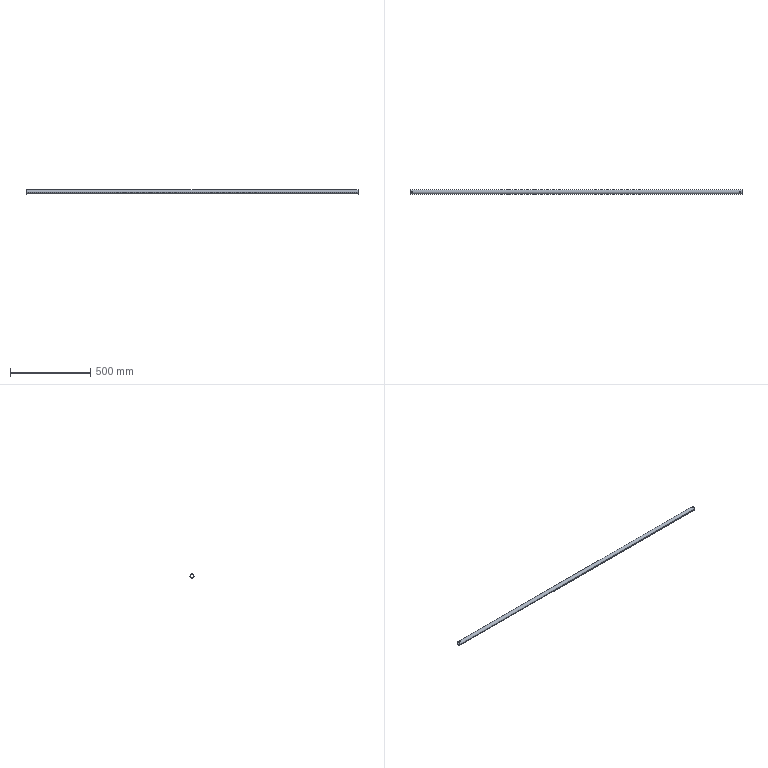Part | NX | features BREP 1 | 1 solid | 10 faces | box 2065 x 25.4 x 25.4 mm | volume 191174 mm3 | cylinder 8 | plane 2 | commonest cylinder face diameters 6.604 x4 22.962 x2 25.4 x2
STEP:
#1=CARTESIAN_POINT('',(-1032.51,12.7,0.));
#2=VERTEX_POINT('',#1);
#3=CARTESIAN_POINT('',(-1032.51,-12.7,0.));
#4=VERTEX_POINT('',#3);
#5=CARTESIAN_POINT('',(-1032.51,0.,0.));
#6=DIRECTION('',(1.,0.,0.));
#7=DIRECTION('',(0.,1.,0.));
#8=AXIS2_PLACEMENT_3D('',#5,#6,#7);
#9=CIRCLE('',#8,12.7);
#10=EDGE_CURVE('',#2,#4,#9,.T.);
#11=ORIENTED_EDGE('',*,*,#10,.F.);
#12=CARTESIAN_POINT('',(-1032.51,0.,0.));
#13=DIRECTION('',(1.,0.,0.));
#14=DIRECTION('',(0.,-1.,0.));
#15=AXIS2_PLACEMENT_3D('',#12,#13,#14);
#16=CIRCLE('',#15,12.7);
#17=EDGE_CURVE('',#4,#2,#16,.T.);
#18=ORIENTED_EDGE('',*,*,#17,.F.);
#19=EDGE_LOOP('',(#11,#18));
#20=FACE_BOUND('',#19,.T.);
#21=CARTESIAN_POINT('',(-1032.51,11.481,0.));
#22=VERTEX_POINT('',#21);
#23=CARTESIAN_POINT('',(-1032.51,-11.481,0.));
#24=VERTEX_POINT('',#23);
#25=CARTESIAN_POINT('',(-1032.51,0.,0.));
#26=DIRECTION('',(-1.,0.,0.));
#27=DIRECTION('',(0.,1.,0.));
#28=AXIS2_PLACEMENT_3D('',#25,#26,#27);
#29=CIRCLE('',#28,11.481);
#30=EDGE_CURVE('',#22,#24,#29,.T.);
#31=ORIENTED_EDGE('',*,*,#30,.F.);
#32=CARTESIAN_POINT('',(-1032.51,0.,0.));
#33=DIRECTION('',(-1.,0.,0.));
#34=DIRECTION('',(0.,-1.,0.));
#35=AXIS2_PLACEMENT_3D('',#32,#33,#34);
#36=CIRCLE('',#35,11.481);
#37=EDGE_CURVE('',#24,#22,#36,.T.);
#38=ORIENTED_EDGE('',*,*,#37,.F.);
#39=EDGE_LOOP('',(#31,#38));
#40=FACE_BOUND('',#39,.T.);
#41=CARTESIAN_POINT('',(-1032.51,0.,0.));
#42=DIRECTION('',(1.,0.,0.));
#43=DIRECTION('',(0.,1.,0.));
#44=AXIS2_PLACEMENT_3D('',#41,#42,#43);
#45=PLANE('',#44);
#46=ADVANCED_FACE('',(#20,#40),#45,.F.);
#47=CARTESIAN_POINT('',(1032.51,12.7,0.));
#48=VERTEX_POINT('',#47);
#49=CARTESIAN_POINT('',(-1032.51,12.7,0.));
#50=DIRECTION('',(1.,0.,0.));
#51=VECTOR('',#50,1000.);
#52=LINE('',#49,#51);
#53=EDGE_CURVE('',#48,#2,#52,.F.);
#54=ORIENTED_EDGE('',*,*,#53,.F.);
#55=CARTESIAN_POINT('',(1032.51,-12.7,0.));
#56=VERTEX_POINT('',#55);
#57=CARTESIAN_POINT('',(1032.51,0.,0.));
#58=DIRECTION('',(1.,0.,0.));
#59=DIRECTION('',(0.,-1.,0.));
#60=AXIS2_PLACEMENT_3D('',#57,#58,#59);
#61=CIRCLE('',#60,12.7);
#62=EDGE_CURVE('',#56,#48,#61,.T.);
#63=ORIENTED_EDGE('',*,*,#62,.F.);
#64=CARTESIAN_POINT('',(-1032.51,-12.7,0.));
#65=DIRECTION('',(1.,0.,0.));
#66=VECTOR('',#65,1000.);
#67=LINE('',#64,#66);
#68=EDGE_CURVE('',#56,#4,#67,.F.);
#69=ORIENTED_EDGE('',*,*,#68,.T.);
#70=ORIENTED_EDGE('',*,*,#17,.T.);
#71=EDGE_LOOP('',(#54,#63,#69,#70));
#72=FACE_BOUND('',#71,.T.);
#73=CARTESIAN_POINT('',(-1032.51,0.,0.));
#74=DIRECTION('',(1.,0.,0.));
#75=DIRECTION('',(0.,-1.,0.));
#76=AXIS2_PLACEMENT_3D('',#73,#74,#75);
#77=CYLINDRICAL_SURFACE('',#76,12.7);
#78=ADVANCED_FACE('',(#72),#77,.T.);
#79=ORIENTED_EDGE('',*,*,#68,.F.);
#80=CARTESIAN_POINT('',(1032.51,0.,0.));
#81=DIRECTION('',(1.,0.,0.));
#82=DIRECTION('',(0.,1.,0.));
#83=AXIS2_PLACEMENT_3D('',#80,#81,#82);
#84=CIRCLE('',#83,12.7);
#85=EDGE_CURVE('',#48,#56,#84,.T.);
#86=ORIENTED_EDGE('',*,*,#85,.F.);
#87=ORIENTED_EDGE('',*,*,#53,.T.);
#88=ORIENTED_EDGE('',*,*,#10,.T.);
#89=EDGE_LOOP('',(#79,#86,#87,#88));
#90=FACE_BOUND('',#89,.T.);
#91=CARTESIAN_POINT('',(1023.112,0.,12.7));
#92=VERTEX_POINT('',#91);
#93=CARTESIAN_POINT('',(1016.508,0.,12.7));
#94=VERTEX_POINT('',#93);
#95=CARTESIAN_POINT('',(1023.112,0.,12.7));
#96=CARTESIAN_POINT('',(1023.112,-0.4503,12.7));
#97=CARTESIAN_POINT('',(1022.958,-1.282,12.655));
#98=CARTESIAN_POINT('',(1021.952,-2.768,12.426));
#99=CARTESIAN_POINT('',(1019.831,-3.655,12.156));
#100=CARTESIAN_POINT('',(1017.67,-2.773,12.425));
#101=CARTESIAN_POINT('',(1016.664,-1.286,12.654));
#102=CARTESIAN_POINT('',(1016.508,-0.4521,12.7));
#103=CARTESIAN_POINT('',(1016.508,0.,12.7));
#104=B_SPLINE_CURVE_WITH_KNOTS('',3,(#95,#96,#97,#98,#99,#100,#101,#102,#103),.UNSPECIFIED.,.F.,.F.,(4,1,1,1,1,1,4),(0.,0.125,0.25,0.5,0.75,0.875,1.),.UNSPECIFIED.);
#105=EDGE_CURVE('',#92,#94,#104,.T.);
#106=ORIENTED_EDGE('',*,*,#105,.T.);
#107=CARTESIAN_POINT('',(1016.508,0.,12.7));
#108=CARTESIAN_POINT('',(1016.508,0.4503,12.7));
#109=CARTESIAN_POINT('',(1016.662,1.282,12.655));
#110=CARTESIAN_POINT('',(1017.668,2.768,12.426));
#111=CARTESIAN_POINT('',(1019.789,3.655,12.156));
#112=CARTESIAN_POINT('',(1021.95,2.773,12.425));
#113=CARTESIAN_POINT('',(1022.956,1.286,12.654));
#114=CARTESIAN_POINT('',(1023.112,0.4521,12.7));
#115=CARTESIAN_POINT('',(1023.112,0.,12.7));
#116=B_SPLINE_CURVE_WITH_KNOTS('',3,(#107,#108,#109,#110,#111,#112,#113,#114,#115),.UNSPECIFIED.,.F.,.F.,(4,1,1,1,1,1,4),(0.,0.125,0.25,0.5,0.75,0.875,1.),.UNSPECIFIED.);
#117=EDGE_CURVE('',#94,#92,#116,.T.);
#118=ORIENTED_EDGE('',*,*,#117,.T.);
#119=EDGE_LOOP('',(#106,#118));
#120=FACE_BOUND('',#119,.T.);
#121=CARTESIAN_POINT('',(-1016.508,0.,12.7));
#122=VERTEX_POINT('',#121);
#123=CARTESIAN_POINT('',(-1023.112,0.,12.7));
#124=VERTEX_POINT('',#123);
#125=CARTESIAN_POINT('',(-1016.508,0.,12.7));
#126=CARTESIAN_POINT('',(-1016.508,-0.4517,12.7));
#127=CARTESIAN_POINT('',(-1016.664,-1.285,12.654));
#128=CARTESIAN_POINT('',(-1017.67,-2.774,12.425));
#129=CARTESIAN_POINT('',(-1019.831,-3.655,12.156));
#130=CARTESIAN_POINT('',(-1021.952,-2.767,12.426));
#131=CARTESIAN_POINT('',(-1022.958,-1.282,12.655));
#132=CARTESIAN_POINT('',(-1023.112,-0.4506,12.7));
#133=CARTESIAN_POINT('',(-1023.112,0.,12.7));
#134=B_SPLINE_CURVE_WITH_KNOTS('',3,(#125,#126,#127,#128,#129,#130,#131,#132,#133),.UNSPECIFIED.,.F.,.F.,(4,1,1,1,1,1,4),(0.,0.125,0.25,0.5,0.75,0.875,1.),.UNSPECIFIED.);
#135=EDGE_CURVE('',#122,#124,#134,.T.);
#136=ORIENTED_EDGE('',*,*,#135,.T.);
#137=CARTESIAN_POINT('',(-1023.112,0.,12.7));
#138=CARTESIAN_POINT('',(-1023.112,0.4517,12.7));
#139=CARTESIAN_POINT('',(-1022.956,1.285,12.654));
#140=CARTESIAN_POINT('',(-1021.95,2.774,12.425));
#141=CARTESIAN_POINT('',(-1019.789,3.655,12.156));
#142=CARTESIAN_POINT('',(-1017.668,2.767,12.426));
#143=CARTESIAN_POINT('',(-1016.662,1.282,12.655));
#144=CARTESIAN_POINT('',(-1016.508,0.4506,12.7));
#145=CARTESIAN_POINT('',(-1016.508,0.,12.7));
#146=B_SPLINE_CURVE_WITH_KNOTS('',3,(#137,#138,#139,#140,#141,#142,#143,#144,#145),.UNSPECIFIED.,.F.,.F.,(4,1,1,1,1,1,4),(0.,0.125,0.25,0.5,0.75,0.875,1.),.UNSPECIFIED.);
#147=EDGE_CURVE('',#124,#122,#146,.T.);
#148=ORIENTED_EDGE('',*,*,#147,.T.);
#149=EDGE_LOOP('',(#136,#148));
#150=FACE_BOUND('',#149,.T.);
#151=CARTESIAN_POINT('',(-1032.51,0.,0.));
#152=DIRECTION('',(1.,0.,0.));
#153=DIRECTION('',(0.,-1.,0.));
#154=AXIS2_PLACEMENT_3D('',#151,#152,#153);
#155=CYLINDRICAL_SURFACE('',#154,12.7);
#156=ADVANCED_FACE('',(#90,#120,#150),#155,.T.);
#157=ORIENTED_EDGE('',*,*,#85,.T.);
#158=ORIENTED_EDGE('',*,*,#62,.T.);
#159=EDGE_LOOP('',(#157,#158));
#160=FACE_BOUND('',#159,.T.);
#161=CARTESIAN_POINT('',(1032.51,11.481,0.));
#162=VERTEX_POINT('',#161);
#163=CARTESIAN_POINT('',(1032.51,-11.481,0.));
#164=VERTEX_POINT('',#163);
#165=CARTESIAN_POINT('',(1032.51,0.,0.));
#166=DIRECTION('',(-1.,0.,0.));
#167=DIRECTION('',(0.,1.,0.));
#168=AXIS2_PLACEMENT_3D('',#165,#166,#167);
#169=CIRCLE('',#168,11.481);
#170=EDGE_CURVE('',#162,#164,#169,.T.);
#171=ORIENTED_EDGE('',*,*,#170,.T.);
#172=CARTESIAN_POINT('',(1032.51,0.,0.));
#173=DIRECTION('',(-1.,0.,0.));
#174=DIRECTION('',(0.,-1.,0.));
#175=AXIS2_PLACEMENT_3D('',#172,#173,#174);
#176=CIRCLE('',#175,11.481);
#177=EDGE_CURVE('',#164,#162,#176,.T.);
#178=ORIENTED_EDGE('',*,*,#177,.T.);
#179=EDGE_LOOP('',(#171,#178));
#180=FACE_BOUND('',#179,.T.);
#181=CARTESIAN_POINT('',(1032.51,0.,0.));
#182=DIRECTION('',(1.,0.,0.));
#183=DIRECTION('',(0.,1.,0.));
#184=AXIS2_PLACEMENT_3D('',#181,#182,#183);
#185=PLANE('',#184);
#186=ADVANCED_FACE('',(#160,#180),#185,.T.);
#187=CARTESIAN_POINT('',(-1032.51,11.481,0.));
#188=DIRECTION('',(1.,0.,0.));
#189=VECTOR('',#188,1000.);
#190=LINE('',#187,#189);
#191=EDGE_CURVE('',#162,#22,#190,.F.);
#192=ORIENTED_EDGE('',*,*,#191,.F.);
#193=ORIENTED_EDGE('',*,*,#177,.F.);
#194=CARTESIAN_POINT('',(-1032.51,-11.481,0.));
#195=DIRECTION('',(1.,0.,0.));
#196=VECTOR('',#195,1000.);
#197=LINE('',#194,#196);
#198=EDGE_CURVE('',#164,#24,#197,.F.);
#199=ORIENTED_EDGE('',*,*,#198,.T.);
#200=ORIENTED_EDGE('',*,*,#37,.T.);
#201=EDGE_LOOP('',(#192,#193,#199,#200));
#202=FACE_BOUND('',#201,.T.);
#203=CARTESIAN_POINT('',(1016.508,0.,11.481));
#204=VERTEX_POINT('',#203);
#205=CARTESIAN_POINT('',(1023.112,0.,11.481));
#206=VERTEX_POINT('',#205);
#207=CARTESIAN_POINT('',(1016.508,0.,11.481));
#208=CARTESIAN_POINT('',(1016.508,-0.4517,11.481));
#209=CARTESIAN_POINT('',(1016.662,-1.288,11.429));
#210=CARTESIAN_POINT('',(1017.425,-2.395,11.242));
#211=CARTESIAN_POINT('',(1018.515,-3.152,11.044));
#212=CARTESIAN_POINT('',(1020.268,-3.462,10.943));
#213=CARTESIAN_POINT('',(1021.95,-2.77,11.176));
#214=CARTESIAN_POINT('',(1022.958,-1.282,11.431));
#215=CARTESIAN_POINT('',(1023.112,-0.4505,11.481));
#216=CARTESIAN_POINT('',(1023.112,0.,11.481));
#217=B_SPLINE_CURVE_WITH_KNOTS('',3,(#207,#208,#209,#210,#211,#212,#213,#214,#215,#216),.UNSPECIFIED.,.F.,.F.,(4,1,1,1,1,1,1,4),(0.,0.125,0.25,0.375,0.5,0.75,0.875,1.),.UNSPECIFIED.);
#218=EDGE_CURVE('',#204,#206,#217,.T.);
#219=ORIENTED_EDGE('',*,*,#218,.T.);
#220=CARTESIAN_POINT('',(1023.112,0.,11.481));
#221=CARTESIAN_POINT('',(1023.112,0.4517,11.481));
#222=CARTESIAN_POINT('',(1022.958,1.288,11.429));
#223=CARTESIAN_POINT('',(1022.195,2.395,11.242));
#224=CARTESIAN_POINT('',(1021.105,3.152,11.044));
#225=CARTESIAN_POINT('',(1019.352,3.462,10.943));
#226=CARTESIAN_POINT('',(1017.67,2.77,11.176));
#227=CARTESIAN_POINT('',(1016.662,1.282,11.431));
#228=CARTESIAN_POINT('',(1016.508,0.4505,11.481));
#229=CARTESIAN_POINT('',(1016.508,0.,11.481));
#230=B_SPLINE_CURVE_WITH_KNOTS('',3,(#220,#221,#222,#223,#224,#225,#226,#227,#228,#229),.UNSPECIFIED.,.F.,.F.,(4,1,1,1,1,1,1,4),(0.,0.125,0.25,0.375,0.5,0.75,0.875,1.),.UNSPECIFIED.);
#231=EDGE_CURVE('',#206,#204,#230,.T.);
#232=ORIENTED_EDGE('',*,*,#231,.T.);
#233=EDGE_LOOP('',(#219,#232));
#234=FACE_BOUND('',#233,.T.);
#235=CARTESIAN_POINT('',(-1023.112,0.,11.481));
#236=VERTEX_POINT('',#235);
#237=CARTESIAN_POINT('',(-1016.508,0.,11.481));
#238=VERTEX_POINT('',#237);
#239=CARTESIAN_POINT('',(-1023.112,0.,11.481));
#240=CARTESIAN_POINT('',(-1023.112,-0.4501,11.481));
#241=CARTESIAN_POINT('',(-1022.958,-1.281,11.431));
#242=CARTESIAN_POINT('',(-1021.95,-2.771,11.176));
#243=CARTESIAN_POINT('',(-1020.267,-3.462,10.943));
#244=CARTESIAN_POINT('',(-1018.517,-3.153,11.043));
#245=CARTESIAN_POINT('',(-1017.424,-2.395,11.243));
#246=CARTESIAN_POINT('',(-1016.663,-1.289,11.429));
#247=CARTESIAN_POINT('',(-1016.508,-0.4521,11.481));
#248=CARTESIAN_POINT('',(-1016.508,0.,11.481));
#249=B_SPLINE_CURVE_WITH_KNOTS('',3,(#239,#240,#241,#242,#243,#244,#245,#246,#247,#248),.UNSPECIFIED.,.F.,.F.,(4,1,1,1,1,1,1,4),(0.,0.125,0.25,0.5,0.625,0.75,0.875,1.),.UNSPECIFIED.);
#250=EDGE_CURVE('',#236,#238,#249,.T.);
#251=ORIENTED_EDGE('',*,*,#250,.T.);
#252=CARTESIAN_POINT('',(-1016.508,0.,11.481));
#253=CARTESIAN_POINT('',(-1016.508,0.4501,11.481));
#254=CARTESIAN_POINT('',(-1016.662,1.281,11.431));
#255=CARTESIAN_POINT('',(-1017.67,2.771,11.176));
#256=CARTESIAN_POINT('',(-1019.353,3.462,10.943));
#257=CARTESIAN_POINT('',(-1021.103,3.153,11.043));
#258=CARTESIAN_POINT('',(-1022.196,2.395,11.243));
#259=CARTESIAN_POINT('',(-1022.957,1.289,11.429));
#260=CARTESIAN_POINT('',(-1023.112,0.4521,11.481));
#261=CARTESIAN_POINT('',(-1023.112,0.,11.481));
#262=B_SPLINE_CURVE_WITH_KNOTS('',3,(#252,#253,#254,#255,#256,#257,#258,#259,#260,#261),.UNSPECIFIED.,.F.,.F.,(4,1,1,1,1,1,1,4),(0.,0.125,0.25,0.5,0.625,0.75,0.875,1.),.UNSPECIFIED.);
#263=EDGE_CURVE('',#238,#236,#262,.T.);
#264=ORIENTED_EDGE('',*,*,#263,.T.);
#265=EDGE_LOOP('',(#251,#264));
#266=FACE_BOUND('',#265,.T.);
#267=CARTESIAN_POINT('',(-1032.51,0.,0.));
#268=DIRECTION('',(1.,0.,0.));
#269=DIRECTION('',(0.,-1.,0.));
#270=AXIS2_PLACEMENT_3D('',#267,#268,#269);
#271=CYLINDRICAL_SURFACE('',#270,11.481);
#272=ADVANCED_FACE('',(#202,#234,#266),#271,.F.);
#273=ORIENTED_EDGE('',*,*,#198,.F.);
#274=ORIENTED_EDGE('',*,*,#170,.F.);
#275=ORIENTED_EDGE('',*,*,#191,.T.);
#276=ORIENTED_EDGE('',*,*,#30,.T.);
#277=EDGE_LOOP('',(#273,#274,#275,#276));
#278=FACE_BOUND('',#277,.T.);
#279=CARTESIAN_POINT('',(-1032.51,0.,0.));
#280=DIRECTION('',(1.,0.,0.));
#281=DIRECTION('',(0.,-1.,0.));
#282=AXIS2_PLACEMENT_3D('',#279,#280,#281);
#283=CYLINDRICAL_SURFACE('',#282,11.481);
#284=ADVANCED_FACE('',(#278),#283,.F.);
#285=CARTESIAN_POINT('',(1016.508,0.,12.7));
#286=DIRECTION('',(0.,0.,-1.));
#287=VECTOR('',#286,1000.);
#288=LINE('',#285,#287);
#289=EDGE_CURVE('',#94,#204,#288,.T.);
#290=ORIENTED_EDGE('',*,*,#289,.T.);
#291=ORIENTED_EDGE('',*,*,#231,.F.);
#292=CARTESIAN_POINT('',(1023.112,0.,12.7));
#293=DIRECTION('',(0.,0.,-1.));
#294=VECTOR('',#293,1000.);
#295=LINE('',#292,#294);
#296=EDGE_CURVE('',#92,#206,#295,.T.);
#297=ORIENTED_EDGE('',*,*,#296,.F.);
#298=ORIENTED_EDGE('',*,*,#117,.F.);
#299=EDGE_LOOP('',(#290,#291,#297,#298));
#300=FACE_BOUND('',#299,.T.);
#301=CARTESIAN_POINT('',(1019.81,0.,12.7));
#302=DIRECTION('',(0.,0.,1.));
#303=DIRECTION('',(1.,0.,0.));
#304=AXIS2_PLACEMENT_3D('',#301,#302,#303);
#305=CYLINDRICAL_SURFACE('',#304,3.302);
#306=ADVANCED_FACE('',(#300),#305,.F.);
#307=ORIENTED_EDGE('',*,*,#296,.T.);
#308=ORIENTED_EDGE('',*,*,#218,.F.);
#309=ORIENTED_EDGE('',*,*,#289,.F.);
#310=ORIENTED_EDGE('',*,*,#105,.F.);
#311=EDGE_LOOP('',(#307,#308,#309,#310));
#312=FACE_BOUND('',#311,.T.);
#313=CARTESIAN_POINT('',(1019.81,0.,12.7));
#314=DIRECTION('',(0.,0.,1.));
#315=DIRECTION('',(1.,0.,0.));
#316=AXIS2_PLACEMENT_3D('',#313,#314,#315);
#317=CYLINDRICAL_SURFACE('',#316,3.302);
#318=ADVANCED_FACE('',(#312),#317,.F.);
#319=CARTESIAN_POINT('',(-1023.112,0.,12.7));
#320=DIRECTION('',(0.,0.,-1.));
#321=VECTOR('',#320,1000.);
#322=LINE('',#319,#321);
#323=EDGE_CURVE('',#124,#236,#322,.T.);
#324=ORIENTED_EDGE('',*,*,#323,.T.);
#325=ORIENTED_EDGE('',*,*,#263,.F.);
#326=CARTESIAN_POINT('',(-1016.508,0.,12.7));
#327=DIRECTION('',(0.,0.,-1.));
#328=VECTOR('',#327,1000.);
#329=LINE('',#326,#328);
#330=EDGE_CURVE('',#122,#238,#329,.T.);
#331=ORIENTED_EDGE('',*,*,#330,.F.);
#332=ORIENTED_EDGE('',*,*,#147,.F.);
#333=EDGE_LOOP('',(#324,#325,#331,#332));
#334=FACE_BOUND('',#333,.T.);
#335=CARTESIAN_POINT('',(-1019.81,0.,12.7));
#336=DIRECTION('',(0.,0.,-1.));
#337=DIRECTION('',(-1.,0.,0.));
#338=AXIS2_PLACEMENT_3D('',#335,#336,#337);
#339=CYLINDRICAL_SURFACE('',#338,3.302);
#340=ADVANCED_FACE('',(#334),#339,.F.);
#341=ORIENTED_EDGE('',*,*,#330,.T.);
#342=ORIENTED_EDGE('',*,*,#250,.F.);
#343=ORIENTED_EDGE('',*,*,#323,.F.);
#344=ORIENTED_EDGE('',*,*,#135,.F.);
#345=EDGE_LOOP('',(#341,#342,#343,#344));
#346=FACE_BOUND('',#345,.T.);
#347=CARTESIAN_POINT('',(-1019.81,0.,12.7));
#348=DIRECTION('',(0.,0.,-1.));
#349=DIRECTION('',(-1.,0.,0.));
#350=AXIS2_PLACEMENT_3D('',#347,#348,#349);
#351=CYLINDRICAL_SURFACE('',#350,3.302);
#352=ADVANCED_FACE('',(#346),#351,.F.);
#353=CLOSED_SHELL('',(#46,#78,#156,#186,#272,#284,#306,#318,#340,#352));
#354=MANIFOLD_SOLID_BREP('',#353);
#355=(LENGTH_UNIT()NAMED_UNIT(*)SI_UNIT(.MILLI.,.METRE.));
#356=UNCERTAINTY_MEASURE_WITH_UNIT(LENGTH_MEASURE(0.0508),#355,'','');
#357=(NAMED_UNIT(*)PLANE_ANGLE_UNIT()SI_UNIT($,.RADIAN.));
#358=(NAMED_UNIT(*)SI_UNIT($,.STERADIAN.)SOLID_ANGLE_UNIT());
#359=(GEOMETRIC_REPRESENTATION_CONTEXT(3)GLOBAL_UNCERTAINTY_ASSIGNED_CONTEXT((#356))GLOBAL_UNIT_ASSIGNED_CONTEXT((#355,#357,#358))REPRESENTATION_CONTEXT('',''));
#360=ADVANCED_BREP_SHAPE_REPRESENTATION('',(#354),#359);